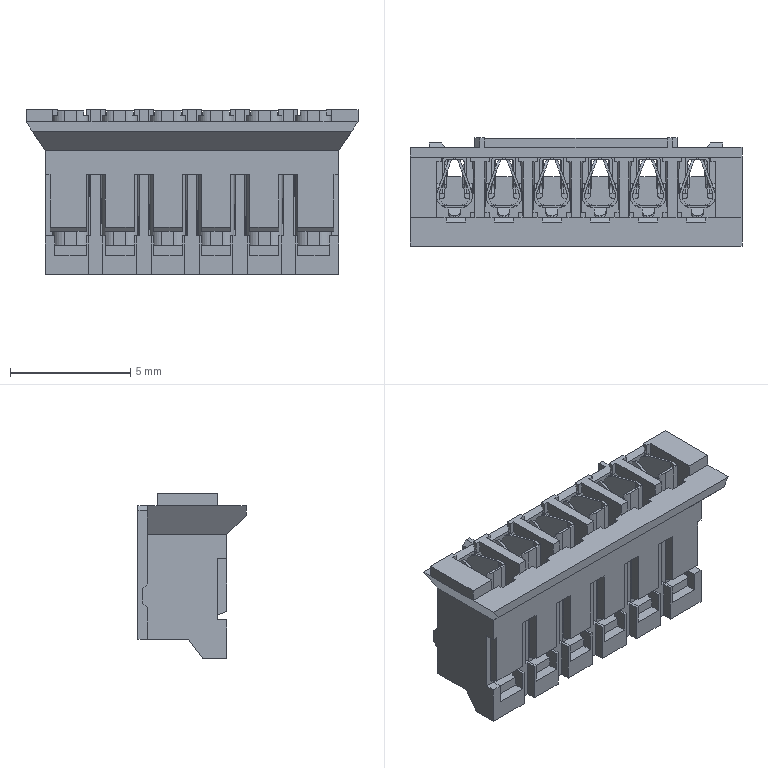Part | NX | features BREP 7 | 7 solids | 1116 faces | box 13.8 x 4.5 x 6.85 mm | volume 132.945 mm3 | plane 690 | cylinder 318 | torus 96 | spline 12 | commonest cylinder face diameters 0.2 x114 0.1 x84 0.4 x72 1 x36 0.8 x12